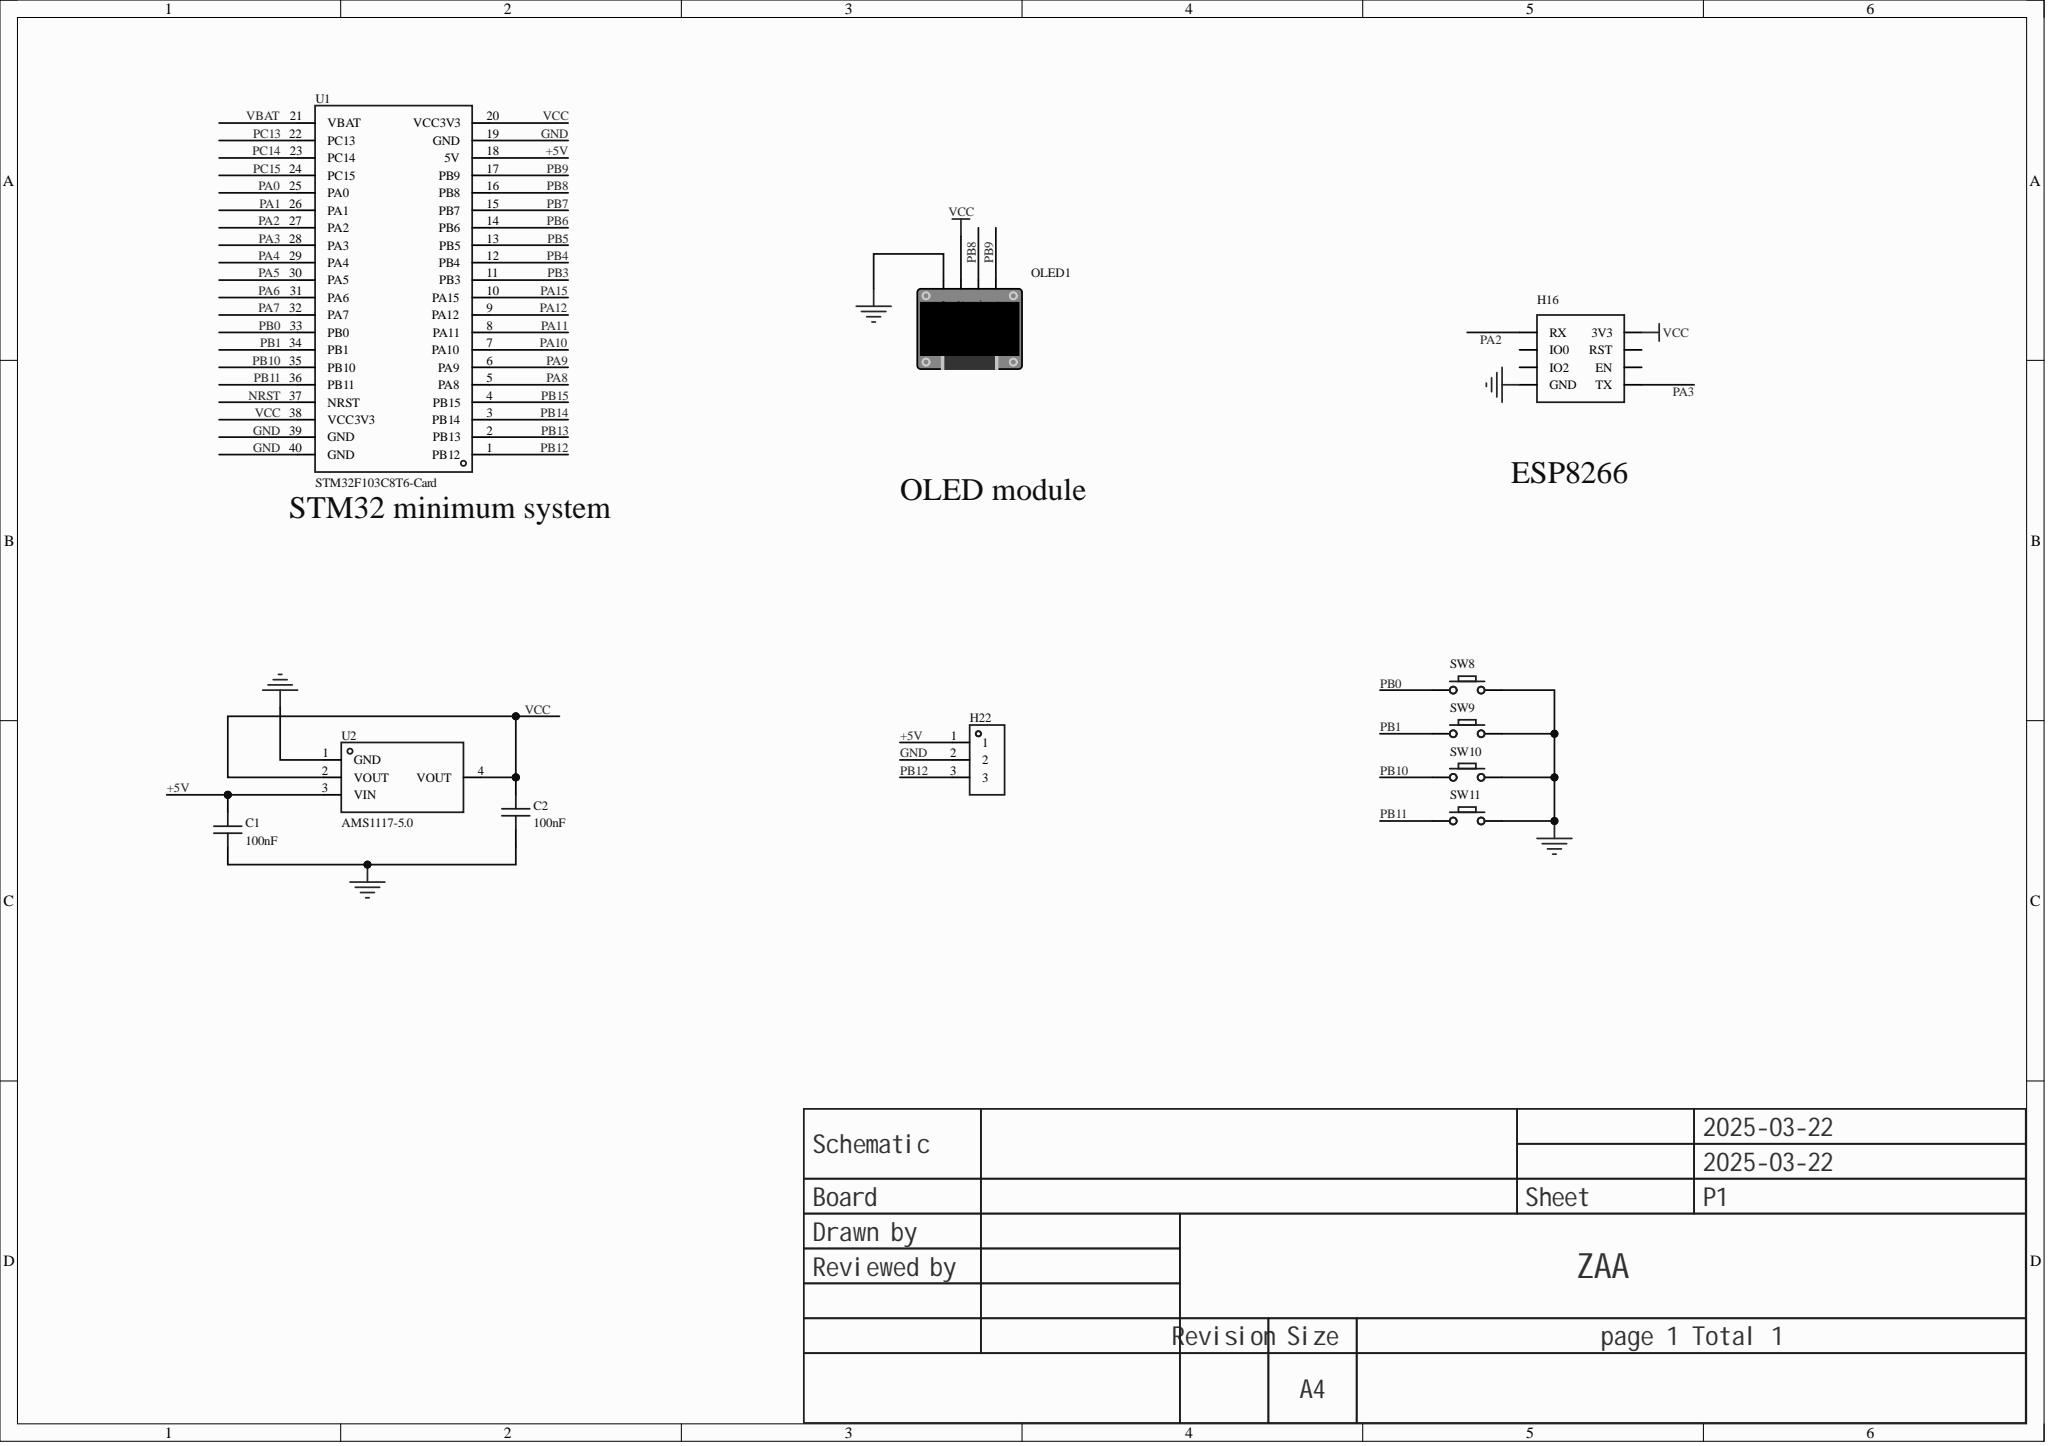Circuit board | Altium Designer | 11 parts | 12 nets
Bill of materials:
Comment,Description,Designator,Footprint,LibRef,Quantity
"100nF","","C1, C2","C0603","CAP_0603","2"
"","","H16","HDR-TH_8P-P2.54-V-F-R2-C4-S2.54-1","HDR-F_2.54_2x4","1"
"","","H22","HDR-TH_3P-P2.54-V-F","HDR-F_2.54_1x3P","1"
"","","OLED1","0.96OLED_4P","0.96OLED模块_4P","1"
"","","SW8, SW9, SW10, SW11","Key_TH_3.5x6x4.3","Key_TH_3.5x6x4.3","4"
"STM32F103C8T6-Card","","U1","CONN-TH_L53.3-W22.9_STM32F103C8T6-CARD","STM32F103C8T6-Card","1"
"AMS1117-5.0","输出类型:固定;工作电压:12V;输出电压:5V;输出电流:1A;电源纹波抑制比(PSRR):-;输出极性:正极;","U2","SOT-223_L6.5-W3.5-P2.30-LS7.0-BR","AMS1117-5.0_C6187","1"
Netlist (Protel format):
[
C1
C0603
100nF



]
[
C2
C0603
100nF



]
[
H16
HDR-TH_8P-P2.54-V-F-R2-C4-S2.54-1




]
[
H22
HDR-TH_3P-P2.54-V-F




]
[
OLED1
0.96OLED_4P




]
[
SW8
Key_TH_3.5x6x4.3




]
[
SW9
Key_TH_3.5x6x4.3




]
[
SW10
Key_TH_3.5x6x4.3




]
[
SW11
Key_TH_3.5x6x4.3




]
[
U1
CONN-TH_L53.3-W22.9_STM32F103C8T6-CARD
STM32F103C8T6-Card



]
[
U2
SOT-223_L6.5-W3.5-P2.30-LS7.0-BR
AMS1117-5.0



]
(
VCC
C2-2
H16-7
OLED1-2
U1-20
U1-38
U2-2
U2-4
)
(
PB12
H22-3
U1-1
)
(
PB11
SW11-A
U1-36
)
(
PB10
SW10-A
U1-35
)
(
PB9
OLED1-4
U1-17
)
(
PB8
OLED1-3
U1-16
)
(
PB1
SW9-A
U1-34
)
(
PB0
SW8-A
U1-33
)
(
PA3
H16-1
U1-28
)
(
PA2
H16-8
U1-27
)
(
GND
C1-1
C2-1
H16-2
H22-2
OLED1-1
SW8-B
SW9-B
SW10-B
SW11-B
U1-19
U1-39
U1-40
U2-1
)
(
+5V
C1-2
H22-1
U1-18
U2-3
)